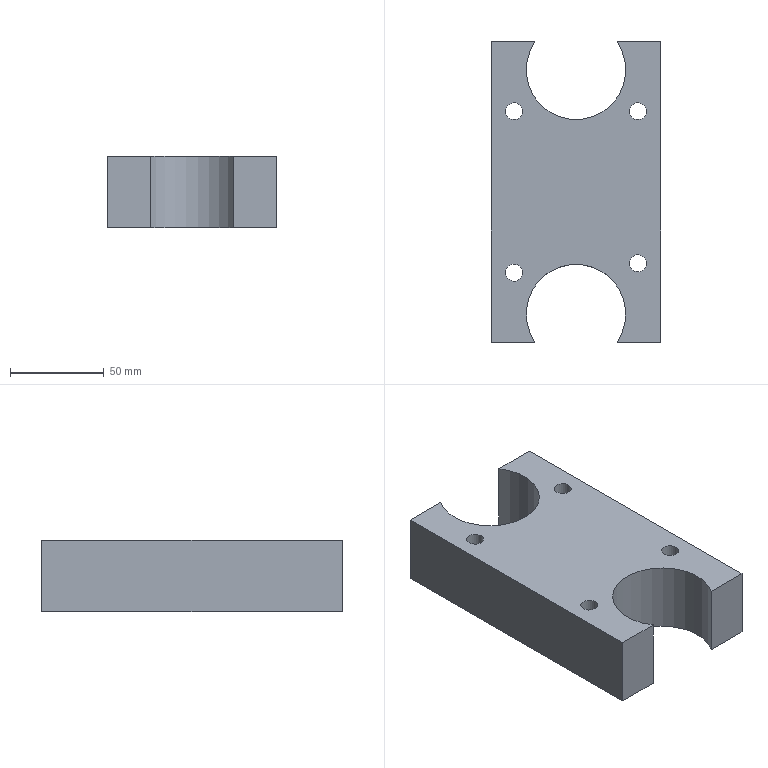Part | NX | features solid 2 | 1 solid | 22 faces | box 90 x 160 x 38 mm | volume 389347 mm3 | plane 12 | cylinder 10 | commonest cylinder face diameters 9.009 x4 14.507 x4 53 x2
STEP:
#1=CARTESIAN_POINT('',(634.5,-80.,50.));
#2=VERTEX_POINT('',#1);
#3=CARTESIAN_POINT('',(634.5,-80.,88.));
#4=VERTEX_POINT('',#3);
#5=CARTESIAN_POINT('',(634.5,-80.,31.));
#6=DIRECTION('',(0.,0.,1.));
#7=VECTOR('',#6,1000.);
#8=LINE('',#5,#7);
#9=EDGE_CURVE('',#2,#4,#8,.T.);
#10=ORIENTED_EDGE('',*,*,#9,.F.);
#11=CARTESIAN_POINT('',(657.654,-80.,50.));
#12=VERTEX_POINT('',#11);
#13=CARTESIAN_POINT('',(679.5,-80.,50.));
#14=DIRECTION('',(1.,0.,0.));
#15=VECTOR('',#14,1000.);
#16=LINE('',#13,#15);
#17=EDGE_CURVE('',#2,#12,#16,.T.);
#18=ORIENTED_EDGE('',*,*,#17,.T.);
#19=CARTESIAN_POINT('',(657.654,-80.,88.));
#20=VERTEX_POINT('',#19);
#21=CARTESIAN_POINT('',(657.654,-80.,148.));
#22=DIRECTION('',(0.,0.,-1.));
#23=VECTOR('',#22,1000.);
#24=LINE('',#21,#23);
#25=EDGE_CURVE('',#20,#12,#24,.T.);
#26=ORIENTED_EDGE('',*,*,#25,.F.);
#27=CARTESIAN_POINT('',(679.5,-80.,88.));
#28=DIRECTION('',(-1.,0.,0.));
#29=VECTOR('',#28,1000.);
#30=LINE('',#27,#29);
#31=EDGE_CURVE('',#20,#4,#30,.T.);
#32=ORIENTED_EDGE('',*,*,#31,.T.);
#33=EDGE_LOOP('',(#10,#18,#26,#32));
#34=FACE_BOUND('',#33,.T.);
#35=CARTESIAN_POINT('',(679.5,-80.,31.));
#36=DIRECTION('',(0.,-1.,0.));
#37=DIRECTION('',(0.,0.,-1.));
#38=AXIS2_PLACEMENT_3D('',#35,#36,#37);
#39=PLANE('',#38);
#40=ADVANCED_FACE('',(#34),#39,.T.);
#41=CARTESIAN_POINT('',(724.5,80.,50.));
#42=VERTEX_POINT('',#41);
#43=CARTESIAN_POINT('',(724.5,80.,88.));
#44=VERTEX_POINT('',#43);
#45=CARTESIAN_POINT('',(724.5,80.,31.));
#46=DIRECTION('',(0.,0.,1.));
#47=VECTOR('',#46,1000.);
#48=LINE('',#45,#47);
#49=EDGE_CURVE('',#42,#44,#48,.T.);
#50=ORIENTED_EDGE('',*,*,#49,.F.);
#51=CARTESIAN_POINT('',(701.346,80.,50.));
#52=VERTEX_POINT('',#51);
#53=CARTESIAN_POINT('',(679.5,80.,50.));
#54=DIRECTION('',(-1.,0.,0.));
#55=VECTOR('',#54,1000.);
#56=LINE('',#53,#55);
#57=EDGE_CURVE('',#42,#52,#56,.T.);
#58=ORIENTED_EDGE('',*,*,#57,.T.);
#59=CARTESIAN_POINT('',(701.346,80.,88.));
#60=VERTEX_POINT('',#59);
#61=CARTESIAN_POINT('',(701.346,80.,148.));
#62=DIRECTION('',(0.,0.,-1.));
#63=VECTOR('',#62,1000.);
#64=LINE('',#61,#63);
#65=EDGE_CURVE('',#52,#60,#64,.F.);
#66=ORIENTED_EDGE('',*,*,#65,.T.);
#67=CARTESIAN_POINT('',(679.5,80.,88.));
#68=DIRECTION('',(1.,0.,0.));
#69=VECTOR('',#68,1000.);
#70=LINE('',#67,#69);
#71=EDGE_CURVE('',#60,#44,#70,.T.);
#72=ORIENTED_EDGE('',*,*,#71,.T.);
#73=EDGE_LOOP('',(#50,#58,#66,#72));
#74=FACE_BOUND('',#73,.T.);
#75=CARTESIAN_POINT('',(679.5,80.,31.));
#76=DIRECTION('',(0.,1.,0.));
#77=DIRECTION('',(0.,0.,1.));
#78=AXIS2_PLACEMENT_3D('',#75,#76,#77);
#79=PLANE('',#78);
#80=ADVANCED_FACE('',(#74),#79,.T.);
#81=CARTESIAN_POINT('',(657.654,80.,88.));
#82=VERTEX_POINT('',#81);
#83=CARTESIAN_POINT('',(657.654,80.,50.));
#84=VERTEX_POINT('',#83);
#85=CARTESIAN_POINT('',(657.654,80.,148.));
#86=DIRECTION('',(0.,0.,-1.));
#87=VECTOR('',#86,1000.);
#88=LINE('',#85,#87);
#89=EDGE_CURVE('',#82,#84,#88,.T.);
#90=ORIENTED_EDGE('',*,*,#89,.T.);
#91=CARTESIAN_POINT('',(634.5,80.,50.));
#92=VERTEX_POINT('',#91);
#93=CARTESIAN_POINT('',(679.5,80.,50.));
#94=DIRECTION('',(-1.,0.,0.));
#95=VECTOR('',#94,1000.);
#96=LINE('',#93,#95);
#97=EDGE_CURVE('',#84,#92,#96,.T.);
#98=ORIENTED_EDGE('',*,*,#97,.T.);
#99=CARTESIAN_POINT('',(634.5,80.,88.));
#100=VERTEX_POINT('',#99);
#101=CARTESIAN_POINT('',(634.5,80.,31.));
#102=DIRECTION('',(0.,0.,1.));
#103=VECTOR('',#102,1000.);
#104=LINE('',#101,#103);
#105=EDGE_CURVE('',#92,#100,#104,.T.);
#106=ORIENTED_EDGE('',*,*,#105,.T.);
#107=CARTESIAN_POINT('',(679.5,80.,88.));
#108=DIRECTION('',(1.,0.,0.));
#109=VECTOR('',#108,1000.);
#110=LINE('',#107,#109);
#111=EDGE_CURVE('',#100,#82,#110,.T.);
#112=ORIENTED_EDGE('',*,*,#111,.T.);
#113=EDGE_LOOP('',(#90,#98,#106,#112));
#114=FACE_BOUND('',#113,.T.);
#115=CARTESIAN_POINT('',(679.5,80.,31.));
#116=DIRECTION('',(0.,1.,0.));
#117=DIRECTION('',(0.,0.,1.));
#118=AXIS2_PLACEMENT_3D('',#115,#116,#117);
#119=PLANE('',#118);
#120=ADVANCED_FACE('',(#114),#119,.T.);
#121=CARTESIAN_POINT('',(701.346,-80.,50.));
#122=VERTEX_POINT('',#121);
#123=CARTESIAN_POINT('',(701.346,-80.,88.));
#124=VERTEX_POINT('',#123);
#125=CARTESIAN_POINT('',(701.346,-80.,148.));
#126=DIRECTION('',(0.,0.,-1.));
#127=VECTOR('',#126,1000.);
#128=LINE('',#125,#127);
#129=EDGE_CURVE('',#122,#124,#128,.F.);
#130=ORIENTED_EDGE('',*,*,#129,.F.);
#131=CARTESIAN_POINT('',(724.5,-80.,50.));
#132=VERTEX_POINT('',#131);
#133=CARTESIAN_POINT('',(679.5,-80.,50.));
#134=DIRECTION('',(1.,0.,0.));
#135=VECTOR('',#134,1000.);
#136=LINE('',#133,#135);
#137=EDGE_CURVE('',#122,#132,#136,.T.);
#138=ORIENTED_EDGE('',*,*,#137,.T.);
#139=CARTESIAN_POINT('',(724.5,-80.,88.));
#140=VERTEX_POINT('',#139);
#141=CARTESIAN_POINT('',(724.5,-80.,31.));
#142=DIRECTION('',(0.,0.,1.));
#143=VECTOR('',#142,1000.);
#144=LINE('',#141,#143);
#145=EDGE_CURVE('',#132,#140,#144,.T.);
#146=ORIENTED_EDGE('',*,*,#145,.T.);
#147=CARTESIAN_POINT('',(679.5,-80.,88.));
#148=DIRECTION('',(-1.,0.,0.));
#149=VECTOR('',#148,1000.);
#150=LINE('',#147,#149);
#151=EDGE_CURVE('',#140,#124,#150,.T.);
#152=ORIENTED_EDGE('',*,*,#151,.T.);
#153=EDGE_LOOP('',(#130,#138,#146,#152));
#154=FACE_BOUND('',#153,.T.);
#155=CARTESIAN_POINT('',(679.5,-80.,31.));
#156=DIRECTION('',(0.,-1.,0.));
#157=DIRECTION('',(0.,0.,-1.));
#158=AXIS2_PLACEMENT_3D('',#155,#156,#157);
#159=PLANE('',#158);
#160=ADVANCED_FACE('',(#154),#159,.T.);
#161=ORIENTED_EDGE('',*,*,#105,.F.);
#162=CARTESIAN_POINT('',(634.5,0.,50.));
#163=DIRECTION('',(0.,-1.,0.));
#164=VECTOR('',#163,1000.);
#165=LINE('',#162,#164);
#166=EDGE_CURVE('',#92,#2,#165,.T.);
#167=ORIENTED_EDGE('',*,*,#166,.T.);
#168=ORIENTED_EDGE('',*,*,#9,.T.);
#169=CARTESIAN_POINT('',(634.5,0.,88.));
#170=DIRECTION('',(0.,1.,0.));
#171=VECTOR('',#170,1000.);
#172=LINE('',#169,#171);
#173=EDGE_CURVE('',#4,#100,#172,.T.);
#174=ORIENTED_EDGE('',*,*,#173,.T.);
#175=EDGE_LOOP('',(#161,#167,#168,#174));
#176=FACE_BOUND('',#175,.T.);
#177=CARTESIAN_POINT('',(634.5,0.,31.));
#178=DIRECTION('',(-1.,0.,0.));
#179=DIRECTION('',(0.,0.,1.));
#180=AXIS2_PLACEMENT_3D('',#177,#178,#179);
#181=PLANE('',#180);
#182=ADVANCED_FACE('',(#176),#181,.T.);
#183=ORIENTED_EDGE('',*,*,#145,.F.);
#184=CARTESIAN_POINT('',(724.5,0.,50.));
#185=DIRECTION('',(0.,1.,0.));
#186=VECTOR('',#185,1000.);
#187=LINE('',#184,#186);
#188=EDGE_CURVE('',#132,#42,#187,.T.);
#189=ORIENTED_EDGE('',*,*,#188,.T.);
#190=ORIENTED_EDGE('',*,*,#49,.T.);
#191=CARTESIAN_POINT('',(724.5,0.,88.));
#192=DIRECTION('',(0.,-1.,0.));
#193=VECTOR('',#192,1000.);
#194=LINE('',#191,#193);
#195=EDGE_CURVE('',#44,#140,#194,.T.);
#196=ORIENTED_EDGE('',*,*,#195,.T.);
#197=EDGE_LOOP('',(#183,#189,#190,#196));
#198=FACE_BOUND('',#197,.T.);
#199=CARTESIAN_POINT('',(724.5,0.,31.));
#200=DIRECTION('',(1.,0.,0.));
#201=DIRECTION('',(0.,0.,-1.));
#202=AXIS2_PLACEMENT_3D('',#199,#200,#201);
#203=PLANE('',#202);
#204=ADVANCED_FACE('',(#198),#203,.T.);
#205=CARTESIAN_POINT('',(679.5,-65.,50.));
#206=DIRECTION('',(0.,0.,-1.));
#207=DIRECTION('',(-1.,0.,0.));
#208=AXIS2_PLACEMENT_3D('',#205,#206,#207);
#209=CIRCLE('',#208,26.5);
#210=EDGE_CURVE('',#122,#12,#209,.F.);
#211=ORIENTED_EDGE('',*,*,#210,.F.);
#212=ORIENTED_EDGE('',*,*,#129,.T.);
#213=CARTESIAN_POINT('',(679.5,-65.,88.));
#214=DIRECTION('',(0.,0.,1.));
#215=DIRECTION('',(1.,0.,0.));
#216=AXIS2_PLACEMENT_3D('',#213,#214,#215);
#217=CIRCLE('',#216,26.5);
#218=EDGE_CURVE('',#124,#20,#217,.T.);
#219=ORIENTED_EDGE('',*,*,#218,.T.);
#220=ORIENTED_EDGE('',*,*,#25,.T.);
#221=EDGE_LOOP('',(#211,#212,#219,#220));
#222=FACE_BOUND('',#221,.T.);
#223=CARTESIAN_POINT('',(679.5,-65.,148.));
#224=DIRECTION('',(0.,0.,-1.));
#225=DIRECTION('',(-1.,0.,0.));
#226=AXIS2_PLACEMENT_3D('',#223,#224,#225);
#227=CYLINDRICAL_SURFACE('',#226,26.5);
#228=ADVANCED_FACE('',(#222),#227,.F.);
#229=ORIENTED_EDGE('',*,*,#65,.F.);
#230=CARTESIAN_POINT('',(679.5,65.,50.));
#231=DIRECTION('',(0.,0.,-1.));
#232=DIRECTION('',(-1.,0.,0.));
#233=AXIS2_PLACEMENT_3D('',#230,#231,#232);
#234=CIRCLE('',#233,26.5);
#235=EDGE_CURVE('',#52,#84,#234,.T.);
#236=ORIENTED_EDGE('',*,*,#235,.T.);
#237=ORIENTED_EDGE('',*,*,#89,.F.);
#238=CARTESIAN_POINT('',(679.5,65.,88.));
#239=DIRECTION('',(0.,0.,1.));
#240=DIRECTION('',(1.,0.,0.));
#241=AXIS2_PLACEMENT_3D('',#238,#239,#240);
#242=CIRCLE('',#241,26.5);
#243=EDGE_CURVE('',#60,#82,#242,.F.);
#244=ORIENTED_EDGE('',*,*,#243,.F.);
#245=EDGE_LOOP('',(#229,#236,#237,#244));
#246=FACE_BOUND('',#245,.T.);
#247=CARTESIAN_POINT('',(679.5,65.,148.));
#248=DIRECTION('',(0.,0.,-1.));
#249=DIRECTION('',(-1.,0.,0.));
#250=AXIS2_PLACEMENT_3D('',#247,#248,#249);
#251=CYLINDRICAL_SURFACE('',#250,26.5);
#252=ADVANCED_FACE('',(#246),#251,.F.);
#253=CARTESIAN_POINT('',(653.754,-43.,68.));
#254=VERTEX_POINT('',#253);
#255=CARTESIAN_POINT('',(646.5,-43.,68.));
#256=DIRECTION('',(0.,0.,1.));
#257=DIRECTION('',(1.,0.,0.));
#258=AXIS2_PLACEMENT_3D('',#255,#256,#257);
#259=CIRCLE('',#258,7.253);
#260=EDGE_CURVE('',#254,#254,#259,.T.);
#261=ORIENTED_EDGE('',*,*,#260,.T.);
#262=EDGE_LOOP('',(#261));
#263=FACE_BOUND('',#262,.T.);
#264=CARTESIAN_POINT('',(639.246,-43.,50.));
#265=VERTEX_POINT('',#264);
#266=CARTESIAN_POINT('',(646.5,-43.,50.));
#267=DIRECTION('',(0.,0.,-1.));
#268=DIRECTION('',(-1.,0.,0.));
#269=AXIS2_PLACEMENT_3D('',#266,#267,#268);
#270=CIRCLE('',#269,7.253);
#271=EDGE_CURVE('',#265,#265,#270,.F.);
#272=ORIENTED_EDGE('',*,*,#271,.F.);
#273=EDGE_LOOP('',(#272));
#274=FACE_BOUND('',#273,.T.);
#275=CARTESIAN_POINT('',(646.5,-43.,40.));
#276=DIRECTION('',(0.,0.,1.));
#277=DIRECTION('',(1.,0.,0.));
#278=AXIS2_PLACEMENT_3D('',#275,#276,#277);
#279=CYLINDRICAL_SURFACE('',#278,7.253);
#280=ADVANCED_FACE('',(#263,#274),#279,.F.);
#281=CARTESIAN_POINT('',(719.754,43.,68.));
#282=VERTEX_POINT('',#281);
#283=CARTESIAN_POINT('',(712.5,43.,68.));
#284=DIRECTION('',(0.,0.,1.));
#285=DIRECTION('',(1.,0.,0.));
#286=AXIS2_PLACEMENT_3D('',#283,#284,#285);
#287=CIRCLE('',#286,7.253);
#288=EDGE_CURVE('',#282,#282,#287,.T.);
#289=ORIENTED_EDGE('',*,*,#288,.T.);
#290=EDGE_LOOP('',(#289));
#291=FACE_BOUND('',#290,.T.);
#292=CARTESIAN_POINT('',(705.246,43.,50.));
#293=VERTEX_POINT('',#292);
#294=CARTESIAN_POINT('',(712.5,43.,50.));
#295=DIRECTION('',(0.,0.,-1.));
#296=DIRECTION('',(-1.,0.,0.));
#297=AXIS2_PLACEMENT_3D('',#294,#295,#296);
#298=CIRCLE('',#297,7.253);
#299=EDGE_CURVE('',#293,#293,#298,.F.);
#300=ORIENTED_EDGE('',*,*,#299,.F.);
#301=EDGE_LOOP('',(#300));
#302=FACE_BOUND('',#301,.T.);
#303=CARTESIAN_POINT('',(712.5,43.,40.));
#304=DIRECTION('',(0.,0.,1.));
#305=DIRECTION('',(1.,0.,0.));
#306=AXIS2_PLACEMENT_3D('',#303,#304,#305);
#307=CYLINDRICAL_SURFACE('',#306,7.253);
#308=ADVANCED_FACE('',(#291,#302),#307,.F.);
#309=CARTESIAN_POINT('',(719.754,-38.,68.));
#310=VERTEX_POINT('',#309);
#311=CARTESIAN_POINT('',(712.5,-38.,68.));
#312=DIRECTION('',(0.,0.,1.));
#313=DIRECTION('',(1.,0.,0.));
#314=AXIS2_PLACEMENT_3D('',#311,#312,#313);
#315=CIRCLE('',#314,7.253);
#316=EDGE_CURVE('',#310,#310,#315,.T.);
#317=ORIENTED_EDGE('',*,*,#316,.T.);
#318=EDGE_LOOP('',(#317));
#319=FACE_BOUND('',#318,.T.);
#320=CARTESIAN_POINT('',(705.246,-38.,50.));
#321=VERTEX_POINT('',#320);
#322=CARTESIAN_POINT('',(712.5,-38.,50.));
#323=DIRECTION('',(0.,0.,-1.));
#324=DIRECTION('',(-1.,0.,0.));
#325=AXIS2_PLACEMENT_3D('',#322,#323,#324);
#326=CIRCLE('',#325,7.253);
#327=EDGE_CURVE('',#321,#321,#326,.F.);
#328=ORIENTED_EDGE('',*,*,#327,.F.);
#329=EDGE_LOOP('',(#328));
#330=FACE_BOUND('',#329,.T.);
#331=CARTESIAN_POINT('',(712.5,-38.,40.));
#332=DIRECTION('',(0.,0.,1.));
#333=DIRECTION('',(1.,0.,0.));
#334=AXIS2_PLACEMENT_3D('',#331,#332,#333);
#335=CYLINDRICAL_SURFACE('',#334,7.253);
#336=ADVANCED_FACE('',(#319,#330),#335,.F.);
#337=CARTESIAN_POINT('',(653.754,43.,68.));
#338=VERTEX_POINT('',#337);
#339=CARTESIAN_POINT('',(646.5,43.,68.));
#340=DIRECTION('',(0.,0.,1.));
#341=DIRECTION('',(1.,0.,0.));
#342=AXIS2_PLACEMENT_3D('',#339,#340,#341);
#343=CIRCLE('',#342,7.253);
#344=EDGE_CURVE('',#338,#338,#343,.T.);
#345=ORIENTED_EDGE('',*,*,#344,.T.);
#346=EDGE_LOOP('',(#345));
#347=FACE_BOUND('',#346,.T.);
#348=CARTESIAN_POINT('',(639.246,43.,50.));
#349=VERTEX_POINT('',#348);
#350=CARTESIAN_POINT('',(646.5,43.,50.));
#351=DIRECTION('',(0.,0.,-1.));
#352=DIRECTION('',(-1.,0.,0.));
#353=AXIS2_PLACEMENT_3D('',#350,#351,#352);
#354=CIRCLE('',#353,7.253);
#355=EDGE_CURVE('',#349,#349,#354,.F.);
#356=ORIENTED_EDGE('',*,*,#355,.F.);
#357=EDGE_LOOP('',(#356));
#358=FACE_BOUND('',#357,.T.);
#359=CARTESIAN_POINT('',(646.5,43.,40.));
#360=DIRECTION('',(0.,0.,1.));
#361=DIRECTION('',(1.,0.,0.));
#362=AXIS2_PLACEMENT_3D('',#359,#360,#361);
#363=CYLINDRICAL_SURFACE('',#362,7.253);
#364=ADVANCED_FACE('',(#347,#358),#363,.F.);
#365=CARTESIAN_POINT('',(651.005,43.,88.));
#366=VERTEX_POINT('',#365);
#367=CARTESIAN_POINT('',(646.5,43.,88.));
#368=DIRECTION('',(0.,0.,1.));
#369=DIRECTION('',(1.,0.,0.));
#370=AXIS2_PLACEMENT_3D('',#367,#368,#369);
#371=CIRCLE('',#370,4.505);
#372=EDGE_CURVE('',#366,#366,#371,.T.);
#373=ORIENTED_EDGE('',*,*,#372,.F.);
#374=EDGE_LOOP('',(#373));
#375=FACE_BOUND('',#374,.T.);
#376=CARTESIAN_POINT('',(717.005,-38.,88.));
#377=VERTEX_POINT('',#376);
#378=CARTESIAN_POINT('',(712.5,-38.,88.));
#379=DIRECTION('',(0.,0.,1.));
#380=DIRECTION('',(1.,0.,0.));
#381=AXIS2_PLACEMENT_3D('',#378,#379,#380);
#382=CIRCLE('',#381,4.505);
#383=EDGE_CURVE('',#377,#377,#382,.T.);
#384=ORIENTED_EDGE('',*,*,#383,.F.);
#385=EDGE_LOOP('',(#384));
#386=FACE_BOUND('',#385,.T.);
#387=CARTESIAN_POINT('',(717.005,43.,88.));
#388=VERTEX_POINT('',#387);
#389=CARTESIAN_POINT('',(712.5,43.,88.));
#390=DIRECTION('',(0.,0.,1.));
#391=DIRECTION('',(1.,0.,0.));
#392=AXIS2_PLACEMENT_3D('',#389,#390,#391);
#393=CIRCLE('',#392,4.505);
#394=EDGE_CURVE('',#388,#388,#393,.T.);
#395=ORIENTED_EDGE('',*,*,#394,.F.);
#396=EDGE_LOOP('',(#395));
#397=FACE_BOUND('',#396,.T.);
#398=CARTESIAN_POINT('',(651.005,-43.,88.));
#399=VERTEX_POINT('',#398);
#400=CARTESIAN_POINT('',(646.5,-43.,88.));
#401=DIRECTION('',(0.,0.,1.));
#402=DIRECTION('',(1.,0.,0.));
#403=AXIS2_PLACEMENT_3D('',#400,#401,#402);
#404=CIRCLE('',#403,4.505);
#405=EDGE_CURVE('',#399,#399,#404,.T.);
#406=ORIENTED_EDGE('',*,*,#405,.F.);
#407=EDGE_LOOP('',(#406));
#408=FACE_BOUND('',#407,.T.);
#409=ORIENTED_EDGE('',*,*,#71,.F.);
#410=ORIENTED_EDGE('',*,*,#243,.T.);
#411=ORIENTED_EDGE('',*,*,#111,.F.);
#412=ORIENTED_EDGE('',*,*,#173,.F.);
#413=ORIENTED_EDGE('',*,*,#31,.F.);
#414=ORIENTED_EDGE('',*,*,#218,.F.);
#415=ORIENTED_EDGE('',*,*,#151,.F.);
#416=ORIENTED_EDGE('',*,*,#195,.F.);
#417=EDGE_LOOP('',(#409,#410,#411,#412,#413,#414,#415,#416));
#418=FACE_BOUND('',#417,.T.);
#419=CARTESIAN_POINT('',(268.879,0.,88.));
#420=DIRECTION('',(0.,0.,1.));
#421=DIRECTION('',(-1.,0.,0.));
#422=AXIS2_PLACEMENT_3D('',#419,#420,#421);
#423=PLANE('',#422);
#424=ADVANCED_FACE('',(#375,#386,#397,#408,#418),#423,.T.);
#425=ORIENTED_EDGE('',*,*,#405,.T.);
#426=EDGE_LOOP('',(#425));
#427=FACE_BOUND('',#426,.T.);
#428=CARTESIAN_POINT('',(651.005,-43.,68.));
#429=VERTEX_POINT('',#428);
#430=CARTESIAN_POINT('',(646.5,-43.,68.));
#431=DIRECTION('',(0.,0.,1.));
#432=DIRECTION('',(1.,0.,0.));
#433=AXIS2_PLACEMENT_3D('',#430,#431,#432);
#434=CIRCLE('',#433,4.505);
#435=EDGE_CURVE('',#429,#429,#434,.T.);
#436=ORIENTED_EDGE('',*,*,#435,.F.);
#437=EDGE_LOOP('',(#436));
#438=FACE_BOUND('',#437,.T.);
#439=CARTESIAN_POINT('',(646.5,-43.,35.));
#440=DIRECTION('',(0.,0.,1.));
#441=DIRECTION('',(1.,0.,0.));
#442=AXIS2_PLACEMENT_3D('',#439,#440,#441);
#443=CYLINDRICAL_SURFACE('',#442,4.505);
#444=ADVANCED_FACE('',(#427,#438),#443,.F.);
#445=ORIENTED_EDGE('',*,*,#435,.T.);
#446=EDGE_LOOP('',(#445));
#447=FACE_BOUND('',#446,.T.);
#448=ORIENTED_EDGE('',*,*,#260,.F.);
#449=EDGE_LOOP('',(#448));
#450=FACE_BOUND('',#449,.T.);
#451=CARTESIAN_POINT('',(646.5,-43.,68.));
#452=DIRECTION('',(0.,0.,1.));
#453=DIRECTION('',(1.,0.,0.));
#454=AXIS2_PLACEMENT_3D('',#451,#452,#453);
#455=PLANE('',#454);
#456=ADVANCED_FACE('',(#447,#450),#455,.F.);
#457=ORIENTED_EDGE('',*,*,#394,.T.);
#458=EDGE_LOOP('',(#457));
#459=FACE_BOUND('',#458,.T.);
#460=CARTESIAN_POINT('',(717.005,43.,68.));
#461=VERTEX_POINT('',#460);
#462=CARTESIAN_POINT('',(712.5,43.,68.));
#463=DIRECTION('',(0.,0.,1.));
#464=DIRECTION('',(1.,0.,0.));
#465=AXIS2_PLACEMENT_3D('',#462,#463,#464);
#466=CIRCLE('',#465,4.505);
#467=EDGE_CURVE('',#461,#461,#466,.T.);
#468=ORIENTED_EDGE('',*,*,#467,.F.);
#469=EDGE_LOOP('',(#468));
#470=FACE_BOUND('',#469,.T.);
#471=CARTESIAN_POINT('',(712.5,43.,35.));
#472=DIRECTION('',(0.,0.,1.));
#473=DIRECTION('',(1.,0.,0.));
#474=AXIS2_PLACEMENT_3D('',#471,#472,#473);
#475=CYLINDRICAL_SURFACE('',#474,4.505);
#476=ADVANCED_FACE('',(#459,#470),#475,.F.);
#477=ORIENTED_EDGE('',*,*,#467,.T.);
#478=EDGE_LOOP('',(#477));
#479=FACE_BOUND('',#478,.T.);
#480=ORIENTED_EDGE('',*,*,#288,.F.);
#481=EDGE_LOOP('',(#480));
#482=FACE_BOUND('',#481,.T.);
#483=CARTESIAN_POINT('',(712.5,43.,68.));
#484=DIRECTION('',(0.,0.,1.));
#485=DIRECTION('',(1.,0.,0.));
#486=AXIS2_PLACEMENT_3D('',#483,#484,#485);
#487=PLANE('',#486);
#488=ADVANCED_FACE('',(#479,#482),#487,.F.);
#489=ORIENTED_EDGE('',*,*,#383,.T.);
#490=EDGE_LOOP('',(#489));
#491=FACE_BOUND('',#490,.T.);
#492=CARTESIAN_POINT('',(717.005,-38.,68.));
#493=VERTEX_POINT('',#492);
#494=CARTESIAN_POINT('',(712.5,-38.,68.));
#495=DIRECTION('',(0.,0.,1.));
#496=DIRECTION('',(1.,0.,0.));
#497=AXIS2_PLACEMENT_3D('',#494,#495,#496);
#498=CIRCLE('',#497,4.505);
#499=EDGE_CURVE('',#493,#493,#498,.T.);
#500=ORIENTED_EDGE('',*,*,#499,.F.);
#501=EDGE_LOOP('',(#500));
#502=FACE_BOUND('',#501,.T.);
#503=CARTESIAN_POINT('',(712.5,-38.,35.));
#504=DIRECTION('',(0.,0.,1.));
#505=DIRECTION('',(1.,0.,0.));
#506=AXIS2_PLACEMENT_3D('',#503,#504,#505);
#507=CYLINDRICAL_SURFACE('',#506,4.505);
#508=ADVANCED_FACE('',(#491,#502),#507,.F.);
#509=ORIENTED_EDGE('',*,*,#499,.T.);
#510=EDGE_LOOP('',(#509));
#511=FACE_BOUND('',#510,.T.);
#512=ORIENTED_EDGE('',*,*,#316,.F.);
#513=EDGE_LOOP('',(#512));
#514=FACE_BOUND('',#513,.T.);
#515=CARTESIAN_POINT('',(712.5,-38.,68.));
#516=DIRECTION('',(0.,0.,1.));
#517=DIRECTION('',(1.,0.,0.));
#518=AXIS2_PLACEMENT_3D('',#515,#516,#517);
#519=PLANE('',#518);
#520=ADVANCED_FACE('',(#511,#514),#519,.F.);
#521=ORIENTED_EDGE('',*,*,#372,.T.);
#522=EDGE_LOOP('',(#521));
#523=FACE_BOUND('',#522,.T.);
#524=CARTESIAN_POINT('',(651.005,43.,68.));
#525=VERTEX_POINT('',#524);
#526=CARTESIAN_POINT('',(646.5,43.,68.));
#527=DIRECTION('',(0.,0.,1.));
#528=DIRECTION('',(1.,0.,0.));
#529=AXIS2_PLACEMENT_3D('',#526,#527,#528);
#530=CIRCLE('',#529,4.505);
#531=EDGE_CURVE('',#525,#525,#530,.T.);
#532=ORIENTED_EDGE('',*,*,#531,.F.);
#533=EDGE_LOOP('',(#532));
#534=FACE_BOUND('',#533,.T.);
#535=CARTESIAN_POINT('',(646.5,43.,35.));
#536=DIRECTION('',(0.,0.,1.));
#537=DIRECTION('',(1.,0.,0.));
#538=AXIS2_PLACEMENT_3D('',#535,#536,#537);
#539=CYLINDRICAL_SURFACE('',#538,4.505);
#540=ADVANCED_FACE('',(#523,#534),#539,.F.);
#541=ORIENTED_EDGE('',*,*,#531,.T.);
#542=EDGE_LOOP('',(#541));
#543=FACE_BOUND('',#542,.T.);
#544=ORIENTED_EDGE('',*,*,#344,.F.);
#545=EDGE_LOOP('',(#544));
#546=FACE_BOUND('',#545,.T.);
#547=CARTESIAN_POINT('',(646.5,43.,68.));
#548=DIRECTION('',(0.,0.,1.));
#549=DIRECTION('',(1.,0.,0.));
#550=AXIS2_PLACEMENT_3D('',#547,#548,#549);
#551=PLANE('',#550);
#552=ADVANCED_FACE('',(#543,#546),#551,.F.);
#553=ORIENTED_EDGE('',*,*,#271,.T.);
#554=EDGE_LOOP('',(#553));
#555=FACE_BOUND('',#554,.T.);
#556=ORIENTED_EDGE('',*,*,#327,.T.);
#557=EDGE_LOOP('',(#556));
#558=FACE_BOUND('',#557,.T.);
#559=ORIENTED_EDGE('',*,*,#355,.T.);
#560=EDGE_LOOP('',(#559));
#561=FACE_BOUND('',#560,.T.);
#562=ORIENTED_EDGE('',*,*,#299,.T.);
#563=EDGE_LOOP('',(#562));
#564=FACE_BOUND('',#563,.T.);
#565=ORIENTED_EDGE('',*,*,#137,.F.);
#566=ORIENTED_EDGE('',*,*,#210,.T.);
#567=ORIENTED_EDGE('',*,*,#17,.F.);
#568=ORIENTED_EDGE('',*,*,#166,.F.);
#569=ORIENTED_EDGE('',*,*,#97,.F.);
#570=ORIENTED_EDGE('',*,*,#235,.F.);
#571=ORIENTED_EDGE('',*,*,#57,.F.);
#572=ORIENTED_EDGE('',*,*,#188,.F.);
#573=EDGE_LOOP('',(#565,#566,#567,#568,#569,#570,#571,#572));
#574=FACE_BOUND('',#573,.T.);
#575=CARTESIAN_POINT('',(1127.,0.,50.));
#576=DIRECTION('',(0.,0.,-1.));
#577=DIRECTION('',(-1.,0.,0.));
#578=AXIS2_PLACEMENT_3D('',#575,#576,#577);
#579=PLANE('',#578);
#580=ADVANCED_FACE('',(#555,#558,#561,#564,#574),#579,.T.);
#581=CLOSED_SHELL('',(#40,#80,#120,#160,#182,#204,#228,#252,#280,#308,#336,#364,#424,#444,#456,#476,#488,#508,#520,#540,#552,#580));
#582=MANIFOLD_SOLID_BREP('',#581);
#583=(LENGTH_UNIT()NAMED_UNIT(*)SI_UNIT(.MILLI.,.METRE.));
#584=UNCERTAINTY_MEASURE_WITH_UNIT(LENGTH_MEASURE(0.00001),#583,'','');
#585=(NAMED_UNIT(*)PLANE_ANGLE_UNIT()SI_UNIT($,.RADIAN.));
#586=(NAMED_UNIT(*)SI_UNIT($,.STERADIAN.)SOLID_ANGLE_UNIT());
#587=(GEOMETRIC_REPRESENTATION_CONTEXT(3)GLOBAL_UNCERTAINTY_ASSIGNED_CONTEXT((#584))GLOBAL_UNIT_ASSIGNED_CONTEXT((#583,#585,#586))REPRESENTATION_CONTEXT('',''));
#588=ADVANCED_BREP_SHAPE_REPRESENTATION('',(#582),#587);